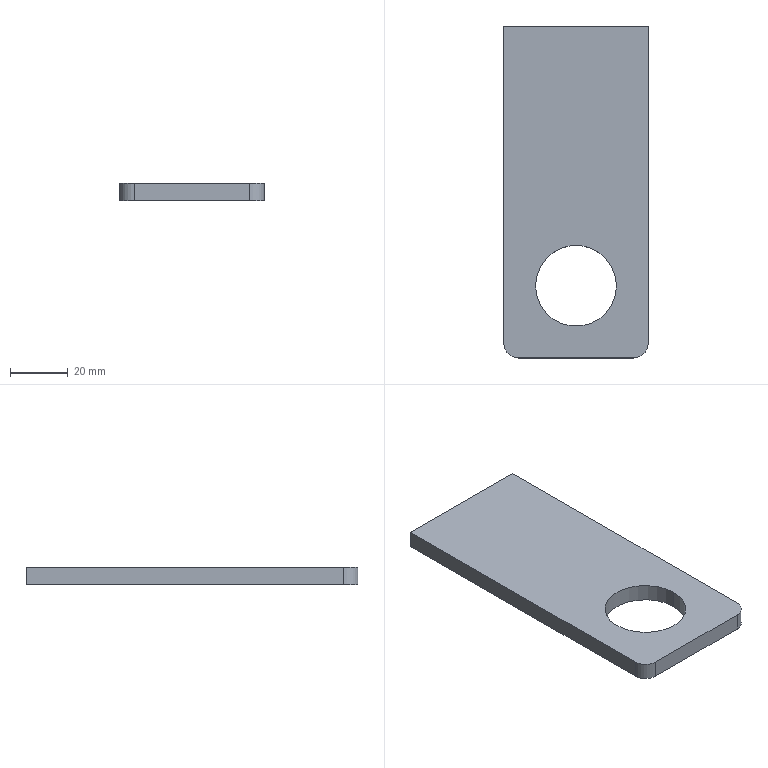Part | SolidWorks | features Extrusion 1 | 1 solid | 10 faces | box 50 x 115 x 6 mm | volume 30741 mm3 | plane 6 | cylinder 4 | commonest cylinder face diameters 10 x2 28 x2
STEP:
#1=CARTESIAN_POINT('',(-14.,0.,3.));
#2=VERTEX_POINT('',#1);
#3=CARTESIAN_POINT('',(14.,0.,3.));
#4=VERTEX_POINT('',#3);
#5=CARTESIAN_POINT('',(0.,0.,3.));
#6=DIRECTION('',(0.,0.,1.));
#7=DIRECTION('',(1.,0.,0.));
#8=AXIS2_PLACEMENT_3D('',#5,#6,#7);
#9=CIRCLE('',#8,14.);
#10=EDGE_CURVE('',#2,#4,#9,.T.);
#11=ORIENTED_EDGE('',*,*,#10,.T.);
#12=CARTESIAN_POINT('',(14.,0.,-3.));
#13=VERTEX_POINT('',#12);
#14=CARTESIAN_POINT('',(14.,0.,3.));
#15=DIRECTION('',(0.,0.,-1.));
#16=VECTOR('',#15,1000.);
#17=LINE('',#14,#16);
#18=EDGE_CURVE('',#4,#13,#17,.T.);
#19=ORIENTED_EDGE('',*,*,#18,.T.);
#20=CARTESIAN_POINT('',(-14.,0.,-3.));
#21=VERTEX_POINT('',#20);
#22=CARTESIAN_POINT('',(0.,0.,-3.));
#23=DIRECTION('',(0.,0.,1.));
#24=DIRECTION('',(1.,0.,0.));
#25=AXIS2_PLACEMENT_3D('',#22,#23,#24);
#26=CIRCLE('',#25,14.);
#27=EDGE_CURVE('',#21,#13,#26,.T.);
#28=ORIENTED_EDGE('',*,*,#27,.F.);
#29=CARTESIAN_POINT('',(-14.,0.,3.));
#30=DIRECTION('',(0.,0.,-1.));
#31=VECTOR('',#30,1000.);
#32=LINE('',#29,#31);
#33=EDGE_CURVE('',#2,#21,#32,.T.);
#34=ORIENTED_EDGE('',*,*,#33,.F.);
#35=EDGE_LOOP('',(#11,#19,#28,#34));
#36=FACE_OUTER_BOUND('',#35,.T.);
#37=CARTESIAN_POINT('',(0.,0.,3.));
#38=DIRECTION('',(0.,0.,-1.));
#39=DIRECTION('',(-1.,0.,0.));
#40=AXIS2_PLACEMENT_3D('',#37,#38,#39);
#41=CYLINDRICAL_SURFACE('',#40,14.);
#42=ADVANCED_FACE('',(#36),#41,.F.);
#43=CARTESIAN_POINT('',(-25.,90.,3.));
#44=VERTEX_POINT('',#43);
#45=CARTESIAN_POINT('',(-25.,-20.,3.));
#46=VERTEX_POINT('',#45);
#47=CARTESIAN_POINT('',(-25.,90.,3.));
#48=DIRECTION('',(0.,-1.,0.));
#49=VECTOR('',#48,1000.);
#50=LINE('',#47,#49);
#51=EDGE_CURVE('',#44,#46,#50,.T.);
#52=ORIENTED_EDGE('',*,*,#51,.T.);
#53=CARTESIAN_POINT('',(-20.,-25.,3.));
#54=VERTEX_POINT('',#53);
#55=CARTESIAN_POINT('',(-20.,-20.,3.));
#56=DIRECTION('',(0.,0.,1.));
#57=DIRECTION('',(1.,0.,0.));
#58=AXIS2_PLACEMENT_3D('',#55,#56,#57);
#59=CIRCLE('',#58,5.);
#60=EDGE_CURVE('',#46,#54,#59,.T.);
#61=ORIENTED_EDGE('',*,*,#60,.T.);
#62=CARTESIAN_POINT('',(20.,-25.,3.));
#63=VERTEX_POINT('',#62);
#64=CARTESIAN_POINT('',(-20.,-25.,3.));
#65=DIRECTION('',(1.,0.,0.));
#66=VECTOR('',#65,1000.);
#67=LINE('',#64,#66);
#68=EDGE_CURVE('',#54,#63,#67,.T.);
#69=ORIENTED_EDGE('',*,*,#68,.T.);
#70=CARTESIAN_POINT('',(25.,-20.,3.));
#71=VERTEX_POINT('',#70);
#72=CARTESIAN_POINT('',(20.,-20.,3.));
#73=DIRECTION('',(0.,0.,1.));
#74=DIRECTION('',(1.,0.,0.));
#75=AXIS2_PLACEMENT_3D('',#72,#73,#74);
#76=CIRCLE('',#75,5.);
#77=EDGE_CURVE('',#63,#71,#76,.T.);
#78=ORIENTED_EDGE('',*,*,#77,.T.);
#79=CARTESIAN_POINT('',(25.,90.,3.));
#80=VERTEX_POINT('',#79);
#81=CARTESIAN_POINT('',(25.,90.,3.));
#82=DIRECTION('',(0.,1.,0.));
#83=VECTOR('',#82,1000.);
#84=LINE('',#81,#83);
#85=EDGE_CURVE('',#71,#80,#84,.T.);
#86=ORIENTED_EDGE('',*,*,#85,.T.);
#87=CARTESIAN_POINT('',(-25.,90.,3.));
#88=DIRECTION('',(-1.,0.,0.));
#89=VECTOR('',#88,1000.);
#90=LINE('',#87,#89);
#91=EDGE_CURVE('',#80,#44,#90,.T.);
#92=ORIENTED_EDGE('',*,*,#91,.T.);
#93=EDGE_LOOP('',(#52,#61,#69,#78,#86,#92));
#94=FACE_OUTER_BOUND('',#93,.T.);
#95=ORIENTED_EDGE('',*,*,#10,.F.);
#96=CARTESIAN_POINT('',(0.,0.,3.));
#97=DIRECTION('',(0.,0.,1.));
#98=DIRECTION('',(1.,0.,0.));
#99=AXIS2_PLACEMENT_3D('',#96,#97,#98);
#100=CIRCLE('',#99,14.);
#101=EDGE_CURVE('',#4,#2,#100,.T.);
#102=ORIENTED_EDGE('',*,*,#101,.F.);
#103=EDGE_LOOP('',(#95,#102));
#104=FACE_BOUND('',#103,.T.);
#105=CARTESIAN_POINT('',(-20.,-20.,3.));
#106=DIRECTION('',(0.,0.,1.));
#107=DIRECTION('',(1.,0.,0.));
#108=AXIS2_PLACEMENT_3D('',#105,#106,#107);
#109=PLANE('',#108);
#110=ADVANCED_FACE('',(#94,#104),#109,.T.);
#111=CARTESIAN_POINT('',(-25.,90.,-3.));
#112=VERTEX_POINT('',#111);
#113=CARTESIAN_POINT('',(-25.,-20.,-3.));
#114=VERTEX_POINT('',#113);
#115=CARTESIAN_POINT('',(-25.,90.,-3.));
#116=DIRECTION('',(0.,-1.,0.));
#117=VECTOR('',#116,1000.);
#118=LINE('',#115,#117);
#119=EDGE_CURVE('',#112,#114,#118,.T.);
#120=ORIENTED_EDGE('',*,*,#119,.F.);
#121=CARTESIAN_POINT('',(25.,90.,-3.));
#122=VERTEX_POINT('',#121);
#123=CARTESIAN_POINT('',(-25.,90.,-3.));
#124=DIRECTION('',(-1.,0.,0.));
#125=VECTOR('',#124,1000.);
#126=LINE('',#123,#125);
#127=EDGE_CURVE('',#122,#112,#126,.T.);
#128=ORIENTED_EDGE('',*,*,#127,.F.);
#129=CARTESIAN_POINT('',(25.,-20.,-3.));
#130=VERTEX_POINT('',#129);
#131=CARTESIAN_POINT('',(25.,90.,-3.));
#132=DIRECTION('',(0.,1.,0.));
#133=VECTOR('',#132,1000.);
#134=LINE('',#131,#133);
#135=EDGE_CURVE('',#130,#122,#134,.T.);
#136=ORIENTED_EDGE('',*,*,#135,.F.);
#137=CARTESIAN_POINT('',(20.,-25.,-3.));
#138=VERTEX_POINT('',#137);
#139=CARTESIAN_POINT('',(20.,-20.,-3.));
#140=DIRECTION('',(0.,0.,1.));
#141=DIRECTION('',(1.,0.,0.));
#142=AXIS2_PLACEMENT_3D('',#139,#140,#141);
#143=CIRCLE('',#142,5.);
#144=EDGE_CURVE('',#138,#130,#143,.T.);
#145=ORIENTED_EDGE('',*,*,#144,.F.);
#146=CARTESIAN_POINT('',(-20.,-25.,-3.));
#147=VERTEX_POINT('',#146);
#148=CARTESIAN_POINT('',(-20.,-25.,-3.));
#149=DIRECTION('',(1.,0.,0.));
#150=VECTOR('',#149,1000.);
#151=LINE('',#148,#150);
#152=EDGE_CURVE('',#147,#138,#151,.T.);
#153=ORIENTED_EDGE('',*,*,#152,.F.);
#154=CARTESIAN_POINT('',(-20.,-20.,-3.));
#155=DIRECTION('',(0.,0.,1.));
#156=DIRECTION('',(1.,0.,0.));
#157=AXIS2_PLACEMENT_3D('',#154,#155,#156);
#158=CIRCLE('',#157,5.);
#159=EDGE_CURVE('',#114,#147,#158,.T.);
#160=ORIENTED_EDGE('',*,*,#159,.F.);
#161=EDGE_LOOP('',(#120,#128,#136,#145,#153,#160));
#162=FACE_OUTER_BOUND('',#161,.T.);
#163=ORIENTED_EDGE('',*,*,#27,.T.);
#164=CARTESIAN_POINT('',(0.,0.,-3.));
#165=DIRECTION('',(0.,0.,1.));
#166=DIRECTION('',(1.,0.,0.));
#167=AXIS2_PLACEMENT_3D('',#164,#165,#166);
#168=CIRCLE('',#167,14.);
#169=EDGE_CURVE('',#13,#21,#168,.T.);
#170=ORIENTED_EDGE('',*,*,#169,.T.);
#171=EDGE_LOOP('',(#163,#170));
#172=FACE_BOUND('',#171,.T.);
#173=CARTESIAN_POINT('',(-20.,-20.,-3.));
#174=DIRECTION('',(0.,0.,1.));
#175=DIRECTION('',(1.,0.,0.));
#176=AXIS2_PLACEMENT_3D('',#173,#174,#175);
#177=PLANE('',#176);
#178=ADVANCED_FACE('',(#162,#172),#177,.F.);
#179=ORIENTED_EDGE('',*,*,#119,.T.);
#180=CARTESIAN_POINT('',(-25.,-20.,3.));
#181=DIRECTION('',(0.,0.,-1.));
#182=VECTOR('',#181,1000.);
#183=LINE('',#180,#182);
#184=EDGE_CURVE('',#46,#114,#183,.T.);
#185=ORIENTED_EDGE('',*,*,#184,.F.);
#186=ORIENTED_EDGE('',*,*,#51,.F.);
#187=CARTESIAN_POINT('',(-25.,90.,3.));
#188=DIRECTION('',(0.,0.,-1.));
#189=VECTOR('',#188,1000.);
#190=LINE('',#187,#189);
#191=EDGE_CURVE('',#44,#112,#190,.T.);
#192=ORIENTED_EDGE('',*,*,#191,.T.);
#193=EDGE_LOOP('',(#179,#185,#186,#192));
#194=FACE_OUTER_BOUND('',#193,.T.);
#195=CARTESIAN_POINT('',(-25.,90.,3.));
#196=DIRECTION('',(1.,0.,0.));
#197=DIRECTION('',(0.,1.,0.));
#198=AXIS2_PLACEMENT_3D('',#195,#196,#197);
#199=PLANE('',#198);
#200=ADVANCED_FACE('',(#194),#199,.F.);
#201=ORIENTED_EDGE('',*,*,#159,.T.);
#202=CARTESIAN_POINT('',(-20.,-25.,3.));
#203=DIRECTION('',(0.,0.,-1.));
#204=VECTOR('',#203,1000.);
#205=LINE('',#202,#204);
#206=EDGE_CURVE('',#54,#147,#205,.T.);
#207=ORIENTED_EDGE('',*,*,#206,.F.);
#208=ORIENTED_EDGE('',*,*,#60,.F.);
#209=ORIENTED_EDGE('',*,*,#184,.T.);
#210=EDGE_LOOP('',(#201,#207,#208,#209));
#211=FACE_OUTER_BOUND('',#210,.T.);
#212=CARTESIAN_POINT('',(-20.,-20.,3.));
#213=DIRECTION('',(0.,0.,-1.));
#214=DIRECTION('',(-1.,0.,0.));
#215=AXIS2_PLACEMENT_3D('',#212,#213,#214);
#216=CYLINDRICAL_SURFACE('',#215,5.);
#217=ADVANCED_FACE('',(#211),#216,.T.);
#218=ORIENTED_EDGE('',*,*,#152,.T.);
#219=CARTESIAN_POINT('',(20.,-25.,3.));
#220=DIRECTION('',(0.,0.,-1.));
#221=VECTOR('',#220,1000.);
#222=LINE('',#219,#221);
#223=EDGE_CURVE('',#63,#138,#222,.T.);
#224=ORIENTED_EDGE('',*,*,#223,.F.);
#225=ORIENTED_EDGE('',*,*,#68,.F.);
#226=ORIENTED_EDGE('',*,*,#206,.T.);
#227=EDGE_LOOP('',(#218,#224,#225,#226));
#228=FACE_OUTER_BOUND('',#227,.T.);
#229=CARTESIAN_POINT('',(-20.,-25.,3.));
#230=DIRECTION('',(0.,1.,0.));
#231=DIRECTION('',(0.,0.,1.));
#232=AXIS2_PLACEMENT_3D('',#229,#230,#231);
#233=PLANE('',#232);
#234=ADVANCED_FACE('',(#228),#233,.F.);
#235=ORIENTED_EDGE('',*,*,#144,.T.);
#236=CARTESIAN_POINT('',(25.,-20.,3.));
#237=DIRECTION('',(0.,0.,-1.));
#238=VECTOR('',#237,1000.);
#239=LINE('',#236,#238);
#240=EDGE_CURVE('',#71,#130,#239,.T.);
#241=ORIENTED_EDGE('',*,*,#240,.F.);
#242=ORIENTED_EDGE('',*,*,#77,.F.);
#243=ORIENTED_EDGE('',*,*,#223,.T.);
#244=EDGE_LOOP('',(#235,#241,#242,#243));
#245=FACE_OUTER_BOUND('',#244,.T.);
#246=CARTESIAN_POINT('',(20.,-20.,3.));
#247=DIRECTION('',(0.,0.,-1.));
#248=DIRECTION('',(-1.,0.,0.));
#249=AXIS2_PLACEMENT_3D('',#246,#247,#248);
#250=CYLINDRICAL_SURFACE('',#249,5.);
#251=ADVANCED_FACE('',(#245),#250,.T.);
#252=ORIENTED_EDGE('',*,*,#135,.T.);
#253=CARTESIAN_POINT('',(25.,90.,3.));
#254=DIRECTION('',(0.,0.,-1.));
#255=VECTOR('',#254,1000.);
#256=LINE('',#253,#255);
#257=EDGE_CURVE('',#80,#122,#256,.T.);
#258=ORIENTED_EDGE('',*,*,#257,.F.);
#259=ORIENTED_EDGE('',*,*,#85,.F.);
#260=ORIENTED_EDGE('',*,*,#240,.T.);
#261=EDGE_LOOP('',(#252,#258,#259,#260));
#262=FACE_OUTER_BOUND('',#261,.T.);
#263=CARTESIAN_POINT('',(25.,90.,3.));
#264=DIRECTION('',(-1.,0.,0.));
#265=DIRECTION('',(0.,-1.,0.));
#266=AXIS2_PLACEMENT_3D('',#263,#264,#265);
#267=PLANE('',#266);
#268=ADVANCED_FACE('',(#262),#267,.F.);
#269=ORIENTED_EDGE('',*,*,#127,.T.);
#270=ORIENTED_EDGE('',*,*,#191,.F.);
#271=ORIENTED_EDGE('',*,*,#91,.F.);
#272=ORIENTED_EDGE('',*,*,#257,.T.);
#273=EDGE_LOOP('',(#269,#270,#271,#272));
#274=FACE_OUTER_BOUND('',#273,.T.);
#275=CARTESIAN_POINT('',(-25.,90.,3.));
#276=DIRECTION('',(0.,-1.,0.));
#277=DIRECTION('',(0.,0.,-1.));
#278=AXIS2_PLACEMENT_3D('',#275,#276,#277);
#279=PLANE('',#278);
#280=ADVANCED_FACE('',(#274),#279,.F.);
#281=ORIENTED_EDGE('',*,*,#18,.F.);
#282=ORIENTED_EDGE('',*,*,#101,.T.);
#283=ORIENTED_EDGE('',*,*,#33,.T.);
#284=ORIENTED_EDGE('',*,*,#169,.F.);
#285=EDGE_LOOP('',(#281,#282,#283,#284));
#286=FACE_OUTER_BOUND('',#285,.T.);
#287=CARTESIAN_POINT('',(0.,0.,3.));
#288=DIRECTION('',(0.,0.,-1.));
#289=DIRECTION('',(-1.,0.,0.));
#290=AXIS2_PLACEMENT_3D('',#287,#288,#289);
#291=CYLINDRICAL_SURFACE('',#290,14.);
#292=ADVANCED_FACE('',(#286),#291,.F.);
#293=CLOSED_SHELL('',(#42,#110,#178,#200,#217,#234,#251,#268,#280,#292));
#294=MANIFOLD_SOLID_BREP('',#293);
#295=CARTESIAN_POINT('',(0.,0.,0.));
#296=DIRECTION('',(0.,0.,1.));
#297=DIRECTION('',(1.,0.,0.));
#298=AXIS2_PLACEMENT_3D('',#295,#296,#297);
#299=(LENGTH_UNIT()NAMED_UNIT(*)SI_UNIT(.MILLI.,.METRE.));
#300=UNCERTAINTY_MEASURE_WITH_UNIT(LENGTH_MEASURE(0.00001),#299,'','');
#301=(NAMED_UNIT(*)PLANE_ANGLE_UNIT()SI_UNIT($,.RADIAN.));
#302=(NAMED_UNIT(*)SI_UNIT($,.STERADIAN.)SOLID_ANGLE_UNIT());
#303=(GEOMETRIC_REPRESENTATION_CONTEXT(3)GLOBAL_UNCERTAINTY_ASSIGNED_CONTEXT((#300))GLOBAL_UNIT_ASSIGNED_CONTEXT((#299,#301,#302))REPRESENTATION_CONTEXT('',''));
#304=ADVANCED_BREP_SHAPE_REPRESENTATION('',(#294,#298),#303);